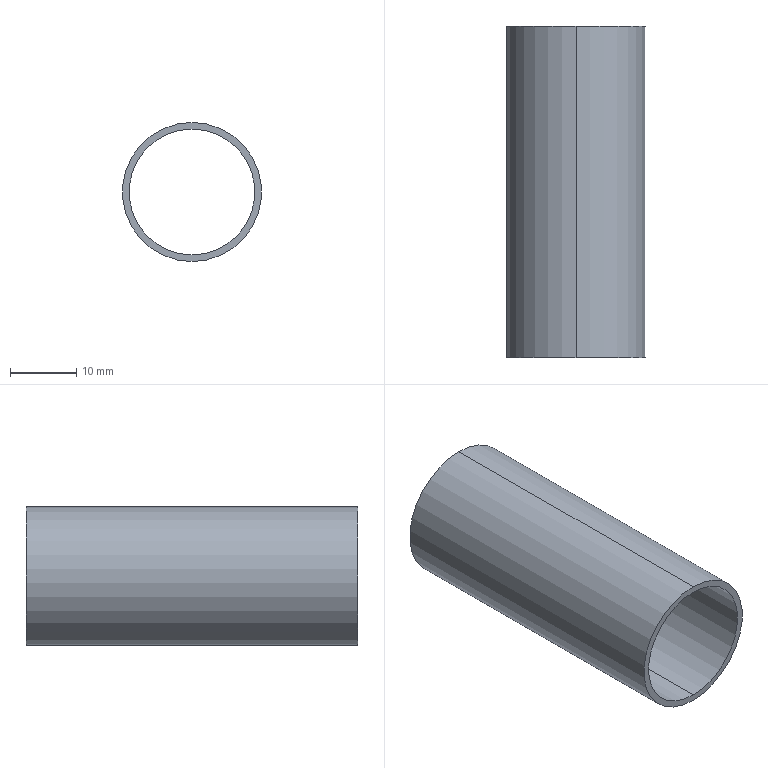Part | SolidWorks | features Extrusion 1 | 1 solid | 6 faces | box 21 x 50 x 21 mm | volume 3142 mm3 | cylinder 4 | plane 2 | commonest cylinder face diameters 19 x2 21 x2
STEP:
#1=CARTESIAN_POINT('',(0.,50.,-9.5));
#2=VERTEX_POINT('',#1);
#3=CARTESIAN_POINT('',(0.,50.,9.5));
#4=VERTEX_POINT('',#3);
#5=CARTESIAN_POINT('',(0.,50.,0.));
#6=DIRECTION('',(0.,1.,0.));
#7=DIRECTION('',(0.,0.,1.));
#8=AXIS2_PLACEMENT_3D('',#5,#6,#7);
#9=CIRCLE('',#8,9.5);
#10=EDGE_CURVE('',#2,#4,#9,.T.);
#11=ORIENTED_EDGE('',*,*,#10,.T.);
#12=CARTESIAN_POINT('',(0.,0.,9.5));
#13=VERTEX_POINT('',#12);
#14=CARTESIAN_POINT('',(0.,50.,9.5));
#15=DIRECTION('',(0.,-1.,0.));
#16=VECTOR('',#15,1000.);
#17=LINE('',#14,#16);
#18=EDGE_CURVE('',#4,#13,#17,.T.);
#19=ORIENTED_EDGE('',*,*,#18,.T.);
#20=CARTESIAN_POINT('',(0.,0.,-9.5));
#21=VERTEX_POINT('',#20);
#22=CARTESIAN_POINT('',(0.,0.,0.));
#23=DIRECTION('',(0.,1.,0.));
#24=DIRECTION('',(0.,0.,1.));
#25=AXIS2_PLACEMENT_3D('',#22,#23,#24);
#26=CIRCLE('',#25,9.5);
#27=EDGE_CURVE('',#21,#13,#26,.T.);
#28=ORIENTED_EDGE('',*,*,#27,.F.);
#29=CARTESIAN_POINT('',(0.,50.,-9.5));
#30=DIRECTION('',(0.,-1.,0.));
#31=VECTOR('',#30,1000.);
#32=LINE('',#29,#31);
#33=EDGE_CURVE('',#2,#21,#32,.T.);
#34=ORIENTED_EDGE('',*,*,#33,.F.);
#35=EDGE_LOOP('',(#11,#19,#28,#34));
#36=FACE_OUTER_BOUND('',#35,.T.);
#37=CARTESIAN_POINT('',(0.,50.,0.));
#38=DIRECTION('',(0.,-1.,0.));
#39=DIRECTION('',(0.,0.,-1.));
#40=AXIS2_PLACEMENT_3D('',#37,#38,#39);
#41=CYLINDRICAL_SURFACE('',#40,9.5);
#42=ADVANCED_FACE('',(#36),#41,.F.);
#43=CARTESIAN_POINT('',(0.,50.,10.5));
#44=VERTEX_POINT('',#43);
#45=CARTESIAN_POINT('',(0.,50.,-10.5));
#46=VERTEX_POINT('',#45);
#47=CARTESIAN_POINT('',(0.,50.,0.));
#48=DIRECTION('',(0.,1.,0.));
#49=DIRECTION('',(0.,0.,1.));
#50=AXIS2_PLACEMENT_3D('',#47,#48,#49);
#51=CIRCLE('',#50,10.5);
#52=EDGE_CURVE('',#44,#46,#51,.T.);
#53=ORIENTED_EDGE('',*,*,#52,.F.);
#54=CARTESIAN_POINT('',(0.,0.,10.5));
#55=VERTEX_POINT('',#54);
#56=CARTESIAN_POINT('',(0.,50.,10.5));
#57=DIRECTION('',(0.,-1.,0.));
#58=VECTOR('',#57,1000.);
#59=LINE('',#56,#58);
#60=EDGE_CURVE('',#44,#55,#59,.T.);
#61=ORIENTED_EDGE('',*,*,#60,.T.);
#62=CARTESIAN_POINT('',(0.,0.,-10.5));
#63=VERTEX_POINT('',#62);
#64=CARTESIAN_POINT('',(0.,0.,0.));
#65=DIRECTION('',(0.,1.,0.));
#66=DIRECTION('',(0.,0.,1.));
#67=AXIS2_PLACEMENT_3D('',#64,#65,#66);
#68=CIRCLE('',#67,10.5);
#69=EDGE_CURVE('',#55,#63,#68,.T.);
#70=ORIENTED_EDGE('',*,*,#69,.T.);
#71=CARTESIAN_POINT('',(0.,50.,-10.5));
#72=DIRECTION('',(0.,-1.,0.));
#73=VECTOR('',#72,1000.);
#74=LINE('',#71,#73);
#75=EDGE_CURVE('',#46,#63,#74,.T.);
#76=ORIENTED_EDGE('',*,*,#75,.F.);
#77=EDGE_LOOP('',(#53,#61,#70,#76));
#78=FACE_OUTER_BOUND('',#77,.T.);
#79=CARTESIAN_POINT('',(0.,50.,0.));
#80=DIRECTION('',(0.,-1.,0.));
#81=DIRECTION('',(0.,0.,-1.));
#82=AXIS2_PLACEMENT_3D('',#79,#80,#81);
#83=CYLINDRICAL_SURFACE('',#82,10.5);
#84=ADVANCED_FACE('',(#78),#83,.T.);
#85=CARTESIAN_POINT('',(0.,50.,0.));
#86=DIRECTION('',(0.,1.,0.));
#87=DIRECTION('',(0.,0.,1.));
#88=AXIS2_PLACEMENT_3D('',#85,#86,#87);
#89=CIRCLE('',#88,10.5);
#90=EDGE_CURVE('',#46,#44,#89,.T.);
#91=ORIENTED_EDGE('',*,*,#90,.T.);
#92=ORIENTED_EDGE('',*,*,#52,.T.);
#93=EDGE_LOOP('',(#91,#92));
#94=FACE_OUTER_BOUND('',#93,.T.);
#95=ORIENTED_EDGE('',*,*,#10,.F.);
#96=CARTESIAN_POINT('',(0.,50.,0.));
#97=DIRECTION('',(0.,1.,0.));
#98=DIRECTION('',(0.,0.,1.));
#99=AXIS2_PLACEMENT_3D('',#96,#97,#98);
#100=CIRCLE('',#99,9.5);
#101=EDGE_CURVE('',#4,#2,#100,.T.);
#102=ORIENTED_EDGE('',*,*,#101,.F.);
#103=EDGE_LOOP('',(#95,#102));
#104=FACE_BOUND('',#103,.T.);
#105=CARTESIAN_POINT('',(0.,50.,0.));
#106=DIRECTION('',(0.,1.,0.));
#107=DIRECTION('',(0.,0.,1.));
#108=AXIS2_PLACEMENT_3D('',#105,#106,#107);
#109=PLANE('',#108);
#110=ADVANCED_FACE('',(#94,#104),#109,.T.);
#111=CARTESIAN_POINT('',(0.,0.,0.));
#112=DIRECTION('',(0.,1.,0.));
#113=DIRECTION('',(0.,0.,1.));
#114=AXIS2_PLACEMENT_3D('',#111,#112,#113);
#115=CIRCLE('',#114,10.5);
#116=EDGE_CURVE('',#63,#55,#115,.T.);
#117=ORIENTED_EDGE('',*,*,#116,.F.);
#118=ORIENTED_EDGE('',*,*,#69,.F.);
#119=EDGE_LOOP('',(#117,#118));
#120=FACE_OUTER_BOUND('',#119,.T.);
#121=ORIENTED_EDGE('',*,*,#27,.T.);
#122=CARTESIAN_POINT('',(0.,0.,0.));
#123=DIRECTION('',(0.,1.,0.));
#124=DIRECTION('',(0.,0.,1.));
#125=AXIS2_PLACEMENT_3D('',#122,#123,#124);
#126=CIRCLE('',#125,9.5);
#127=EDGE_CURVE('',#13,#21,#126,.T.);
#128=ORIENTED_EDGE('',*,*,#127,.T.);
#129=EDGE_LOOP('',(#121,#128));
#130=FACE_BOUND('',#129,.T.);
#131=CARTESIAN_POINT('',(0.,0.,0.));
#132=DIRECTION('',(0.,1.,0.));
#133=DIRECTION('',(0.,0.,1.));
#134=AXIS2_PLACEMENT_3D('',#131,#132,#133);
#135=PLANE('',#134);
#136=ADVANCED_FACE('',(#120,#130),#135,.F.);
#137=ORIENTED_EDGE('',*,*,#60,.F.);
#138=ORIENTED_EDGE('',*,*,#90,.F.);
#139=ORIENTED_EDGE('',*,*,#75,.T.);
#140=ORIENTED_EDGE('',*,*,#116,.T.);
#141=EDGE_LOOP('',(#137,#138,#139,#140));
#142=FACE_OUTER_BOUND('',#141,.T.);
#143=CARTESIAN_POINT('',(0.,50.,0.));
#144=DIRECTION('',(0.,-1.,0.));
#145=DIRECTION('',(0.,0.,-1.));
#146=AXIS2_PLACEMENT_3D('',#143,#144,#145);
#147=CYLINDRICAL_SURFACE('',#146,10.5);
#148=ADVANCED_FACE('',(#142),#147,.T.);
#149=ORIENTED_EDGE('',*,*,#18,.F.);
#150=ORIENTED_EDGE('',*,*,#101,.T.);
#151=ORIENTED_EDGE('',*,*,#33,.T.);
#152=ORIENTED_EDGE('',*,*,#127,.F.);
#153=EDGE_LOOP('',(#149,#150,#151,#152));
#154=FACE_OUTER_BOUND('',#153,.T.);
#155=CARTESIAN_POINT('',(0.,50.,0.));
#156=DIRECTION('',(0.,-1.,0.));
#157=DIRECTION('',(0.,0.,-1.));
#158=AXIS2_PLACEMENT_3D('',#155,#156,#157);
#159=CYLINDRICAL_SURFACE('',#158,9.5);
#160=ADVANCED_FACE('',(#154),#159,.F.);
#161=CLOSED_SHELL('',(#42,#84,#110,#136,#148,#160));
#162=MANIFOLD_SOLID_BREP('',#161);
#163=CARTESIAN_POINT('',(0.,0.,0.));
#164=DIRECTION('',(0.,0.,1.));
#165=DIRECTION('',(1.,0.,0.));
#166=AXIS2_PLACEMENT_3D('',#163,#164,#165);
#167=(LENGTH_UNIT()NAMED_UNIT(*)SI_UNIT(.MILLI.,.METRE.));
#168=UNCERTAINTY_MEASURE_WITH_UNIT(LENGTH_MEASURE(0.00001),#167,'','');
#169=(NAMED_UNIT(*)PLANE_ANGLE_UNIT()SI_UNIT($,.RADIAN.));
#170=(NAMED_UNIT(*)SI_UNIT($,.STERADIAN.)SOLID_ANGLE_UNIT());
#171=(GEOMETRIC_REPRESENTATION_CONTEXT(3)GLOBAL_UNCERTAINTY_ASSIGNED_CONTEXT((#168))GLOBAL_UNIT_ASSIGNED_CONTEXT((#167,#169,#170))REPRESENTATION_CONTEXT('',''));
#172=ADVANCED_BREP_SHAPE_REPRESENTATION('',(#162,#166),#171);